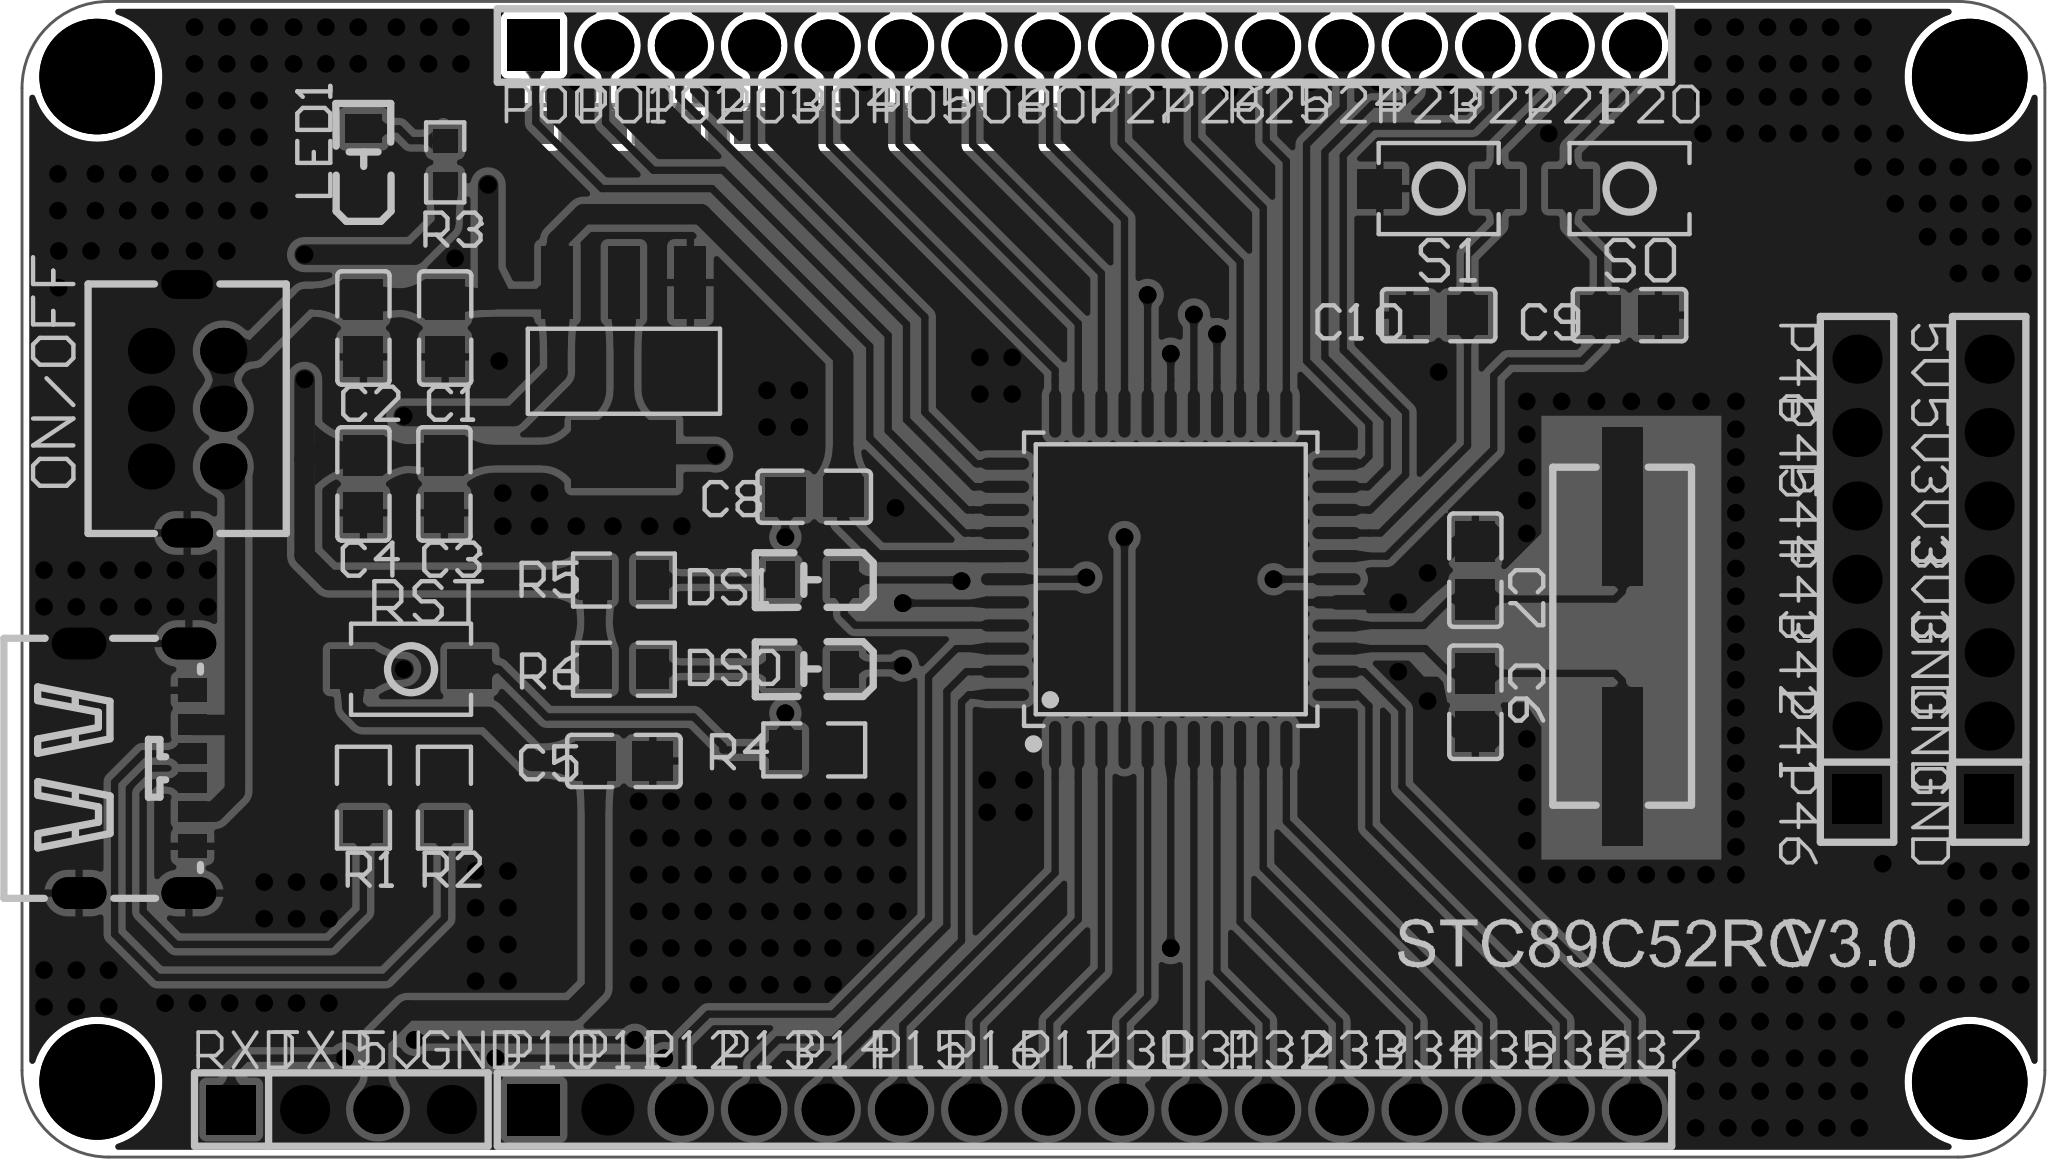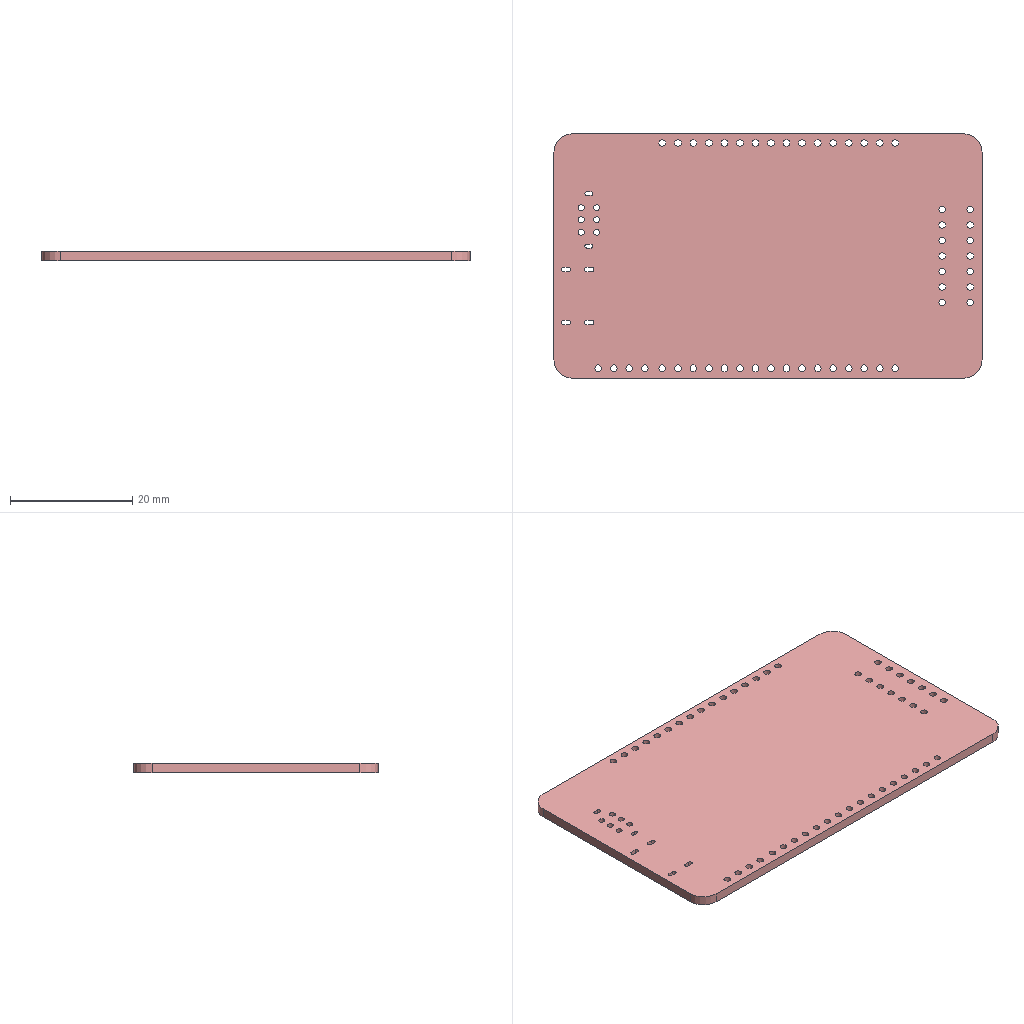Circuit board layout | Altium Designer | box 70 x 40 x 1.6 mm
Layer stack:
# Altium Designer layer stack of  (unit mm; dielectric type: 0 none, 1 core, 2 prepreg, 3 surface material)
index,name,kind,layer,copper_thickness_mm,dielectric_type,dielectric_thickness_mm,dielectric_material,dielectric_constant
0,Top Paste Mask Layer,other,,,,,,
1,Top Silkscreen Layer,other,,,,,,
2,Top Solder Mask Layer,dielectric,,,3,0.01,,3.3
3,Top Layer,copper,Top Layer,0.035,,,,
4,Dielectric1,dielectric,,,3,1.51,FR4,4.5
5,Bottom Layer,copper,Bottom Layer,0.035,,,,
6,Bottom Solder Mask Layer,dielectric,,,3,0.01,,3.3
7,Bottom Silkscreen Layer,other,,,,,,
8,Bottom Paste Mask Layer,other,,,,,,
# drill layer pairs: low layer,high layer
drill_pair,Top Layer,Bottom Layer
Part placement:
Designator,Comment,Layer,Footprint,Center-X(mm),Center-Y(mm),Rotation
USB1,TYPE_C_SMD_6P,TopLayer,TYPE-C-SMD_TYPE-C-6P,82.423,92.837,270
SW2,Tact switch 3*4*H,TopLayer,SW-SMD_L4.0-W2.9-LS5.0,91.948,96.266,180
R1,5.1k,TopLayer,R0805,90.301,91.821,90
C4,10UF,TopLayer,C0805,90.301,102.68,90
C2,10UF,TopLayer,C0805,90.301,108.077,90
LED1,,TopLayer,LED_0805,90.306,113.869,90
R2,5.1k,TopLayer,R0805,93.103,91.821,90
C3,100nF,TopLayer,C0805,93.103,102.68,90
R3,1K,TopLayer,R0603,93.129,113.809,90
C1,100nF,TopLayer,C0805,93.129,108.077,90
U1,AMS1117-3.3,TopLayer,SOT-223-3_L6.5-W3.4-P2.30-LS7.0-BR,99.314,106.68,90
R5,1K,TopLayer,R0805,99.314,99.353,180
R6,1K,TopLayer,R0805,99.314,96.266,180
C5,100nF,TopLayer,C0805,99.314,93.091,180
LED2,,TopLayer,LED_0805,105.841,99.358,180
LED3,,TopLayer,LED_0805,105.841,96.271,180
C8,10UF,TopLayer,C0805,105.901,102.235,180
R4,10K,TopLayer,R0805,105.901,93.472,180
U2,STC89C52RC,TopLayer,LQFP-44_L10.0-W10.0-P0.80-LS12.0-BL,118.237,99.38,0
SW4,Tact switch 3*4*H,TopLayer,SW-SMD_L4.0-W2.9-LS5.0,127.508,112.903,180
C10,10UF,TopLayer,C0805,127.508,108.522,0
C6,47PF,TopLayer,C0805,128.778,95.123,270
C7,47PF,TopLayer,C0805,128.778,99.695,90
SW3,Tact switch 3*4*H,TopLayer,SW-SMD_L4.0-W2.9-LS5.0,134.112,112.903,0
C9,10UF,TopLayer,C0805,134.112,108.522,180
U3,12MHz,TopLayer,CRYSTAL-SMD_L11.4-W4.7-LS12.7,133.858,97.409,270
SW5,SS22D03L6,TopLayer,SW-TH_SS-22D03-L4,84.201,105.283,270
H5,,TopLayer,HDR-TH_4P-P2.54-V-M,89.535,81.026,0
H1,,TopLayer,HDR-TH_16P-P2.54-V-M,115.252,117.856,0
H2,,TopLayer,HDR-TH_16P-P2.54-V-M,115.252,81.026,0
H3,,TopLayer,HDR-TH_7P-P2.54-V-M,141.986,99.377,90
H4,,TopLayer,HDR-TH_7P-P2.54-V-M,146.558,99.377,90
R7,10K,BottomLayer,R0805,96.203,114.029,90
R8,10K,BottomLayer,R0805,98.743,114.029,90
R9,10K,BottomLayer,R0805,101.282,114.029,90
R10,10K,BottomLayer,R0805,103.823,114.029,90
R12,10K,BottomLayer,R0805,106.362,114.029,90
R13,10K,BottomLayer,R0805,108.903,114.029,90
R14,10K,BottomLayer,R0805,111.442,114.029,90
R16,10K,BottomLayer,R0805,113.983,114.029,90
Pad and via stacks:
# Altium Designer via and pad stacks of  (unit mm). Each distinct definition once, with the count of objects using it.
# via: kind,start_layer,end_layer,hole_mm,diameter_mm,mode(0 simple;1 top-mid-bottom;2 full stack),diameter_per_layer,count,example_net
# pad: kind,layer,hole_mm,hole_type(0 round;1 square;2 slot),plating,top_size,top_shape(1 round;2 rect;3 octagon;9 rounded rect),mid_size,bottom_size,mode,footprint,size_per_layer,count,example
pad,Top Layer,0,0,plated,0.8x1,2,0.8x1,0.8x1,0,TYPE-C-SMD_TYPE-C-6P,,2,USB1.B12
pad,Top Layer,0,0,plated,0.7x1,2,0.7x1,0.7x1,0,TYPE-C-SMD_TYPE-C-6P,,4,USB1.B9
pad,Top Layer,0,0,plated,1.53x1.36,2,1.53x1.36,1.53x1.36,0,SW-SMD_L4.0-W2.9-LS5.0,,6,SW2.1
pad,Top Layer,0,0,plated,1.133x1.377,2,1.133x1.377,1.133x1.377,0,R0805,,10,R1.2
pad,Top Layer,0,0,plated,1.41x1.35,2,1.41x1.35,1.41x1.35,0,C0805,,20,C4.2
pad,Top Layer,0,0,plated,1x1.25,2,1x1.25,1x1.25,0,LED_0805,,6,LED1.2
pad,Top Layer,0,0,plated,0.8065x0.864,2,0.8065x0.864,0.8065x0.864,0,R0603,,2,R3.2
pad,Top Layer,0,0,plated,2.5x1.1,2,2.5x1.1,2.5x1.1,0,SOT-223-3_L6.5-W3.4-P2.30-LS7.0-BR,,3,U1.1
pad,Top Layer,0,0,plated,2.34x3.6,2,2.34x3.6,2.34x3.6,0,SOT-223-3_L6.5-W3.4-P2.30-LS7.0-BR,,1,U1.4
pad,Top Layer,0,0,plated,0.42x1.67,1,0.42x1.67,0.42x1.67,0,LQFP-44_L10.0-W10.0-P0.80-LS12.0-BL,,22,U2.1
pad,Top Layer,0,0,plated,1.67x0.42,1,1.67x0.42,1.67x0.42,0,LQFP-44_L10.0-W10.0-P0.80-LS12.0-BL,,22,U2.12
pad,Top Layer,0,0,plated,5.5x1.4,2,5.5x1.4,5.5x1.4,0,CRYSTAL-SMD_L11.4-W4.7-LS12.7,,2,U3.2
pad,Multi-Layer,0.7,2,plated,1.1x1.9,1,1.1x1.9,1.1x1.9,0,TYPE-C-SMD_TYPE-C-6P,,4,USB1.7
pad,Multi-Layer,0.6,2,plated,1x1.8,1,1x1.8,1x1.8,0,SW-TH_SS-22D03-L4,,2,SW5.8
pad,Multi-Layer,1,0,plated,1.6x1.6,1,1.6x1.6,1.6x1.6,0,SW-TH_SS-22D03-L4,,6,SW5.6
pad,Multi-Layer,1.1,0,plated,1.7x1.7,2,1.7x1.7,1.7x1.7,0,HDR-TH_4P-P2.54-V-M,,1,H5.1
pad,Multi-Layer,1.1,0,plated,1.7x1.7,1,1.7x1.7,1.7x1.7,0,HDR-TH_4P-P2.54-V-M,,3,H5.2
pad,Multi-Layer,1.1,0,plated,1.8x1.8,2,1.8x1.8,1.8x1.8,0,HDR-TH_16P-P2.54-V-M,,2,H1.1
pad,Multi-Layer,1.1,0,plated,1.8x1.8,1,1.8x1.8,1.8x1.8,0,HDR-TH_16P-P2.54-V-M,,30,H1.2
pad,Multi-Layer,1.1,0,plated,1.7x1.7,2,1.7x1.7,1.7x1.7,0,HDR-TH_7P-P2.54-V-M,,2,H3.1
pad,Multi-Layer,1.1,0,plated,1.7x1.7,1,1.7x1.7,1.7x1.7,0,HDR-TH_7P-P2.54-V-M,,12,H3.2
pad,Bottom Layer,0,0,plated,1.133x1.377,2,1.133x1.377,1.133x1.377,0,R0805,,16,R7.2
via,Top Layer,Bottom Layer,0.3048,0.6096,0,,328,GND
via,Top Layer,Bottom Layer,3,4,0,,4,
Copper pours:
name,layer,net,type(0 solid;1 hatched;2 none)
Top Layer-GND,Top Layer,GND,0
Bottom Layer-GND,Bottom Layer,GND,0
Design rules, without the lines most boards share:
# Altium Designer design rules of  (exported by Altium Designer, unit mm)
# columns: name | kind | enabled | priority | scope1 | scope2 | descriptor | typed fields (field=value)
creepage | 65 | enabled | 1 | All | All | Creepage Distance Constraint =(0mil) (All),(All) |